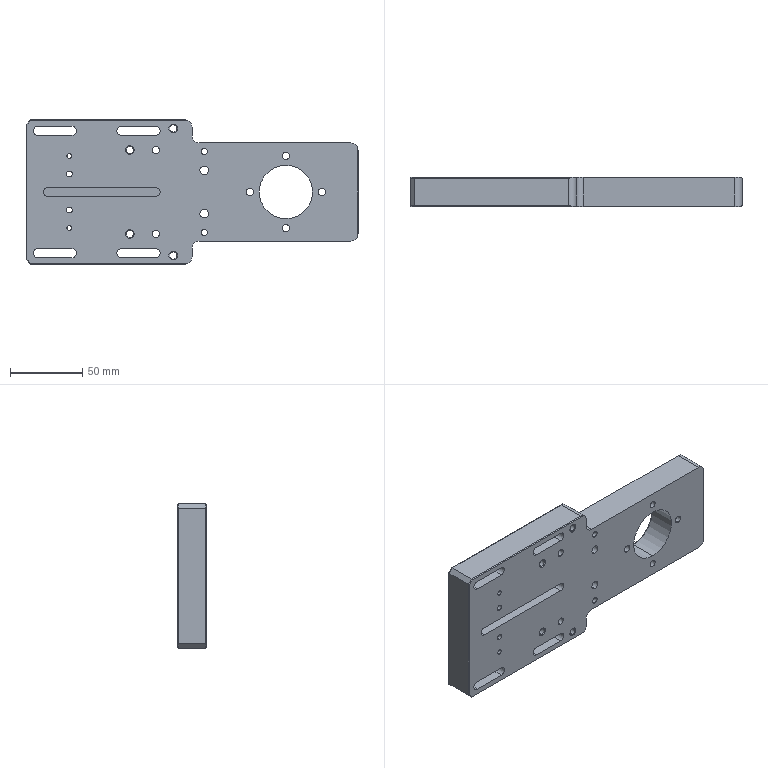Part | SolidWorks | features HoleWzd 11, Chamfer 3, ICE 2, CirPattern 1, Cut 1, Extrusion 1, Fillet 1 | 1 solid | 141 faces | box 230 x 20 x 100 mm | volume 331110 mm3 | cylinder 67 | plane 51 | cone 23 | commonest cylinder face diameters 5 x20 6 x11 6.3 x8 11 x8 10 x6 3.3 x4